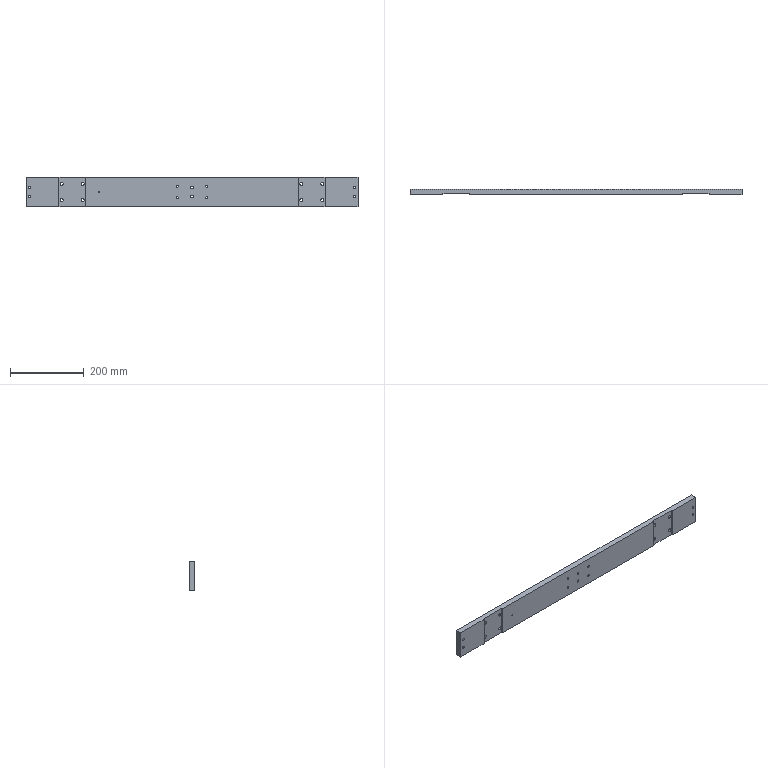Part | SolidWorks | features HoleWzd 4, Extrusion 1, ICE 1, LPattern 1, MirrorPattern 1 | 1 solid | 70 faces | box 900 x 16 x 80 mm | volume 1104727 mm3 | cylinder 50 | plane 20 | commonest cylinder face diameters 8.5 x16 6.6 x12 11 x12 5 x8 4.2 x2